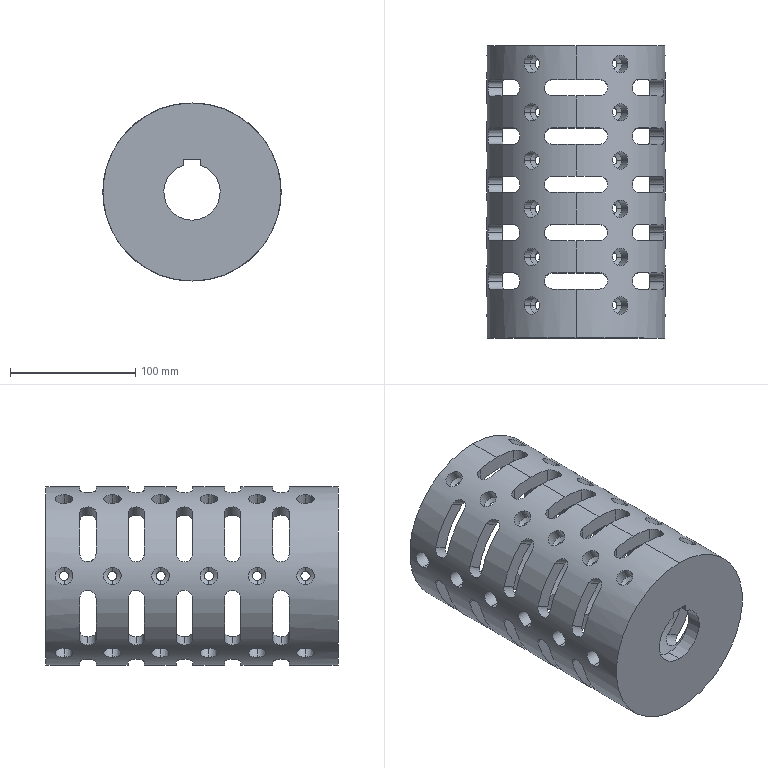Part | SolidWorks | features CirPattern 2, ICE 2, LPattern 2, 3DProfileFeature 1, Extrusion 1, HoleWzd 1 | 1 solid | 311 faces | box 142 x 233 x 142 mm | volume 962955 mm3 | cylinder 173 | cone 72 | plane 66 | commonest cylinder face diameters 13 x95 14 x72 45 x2 118 x2 142 x2